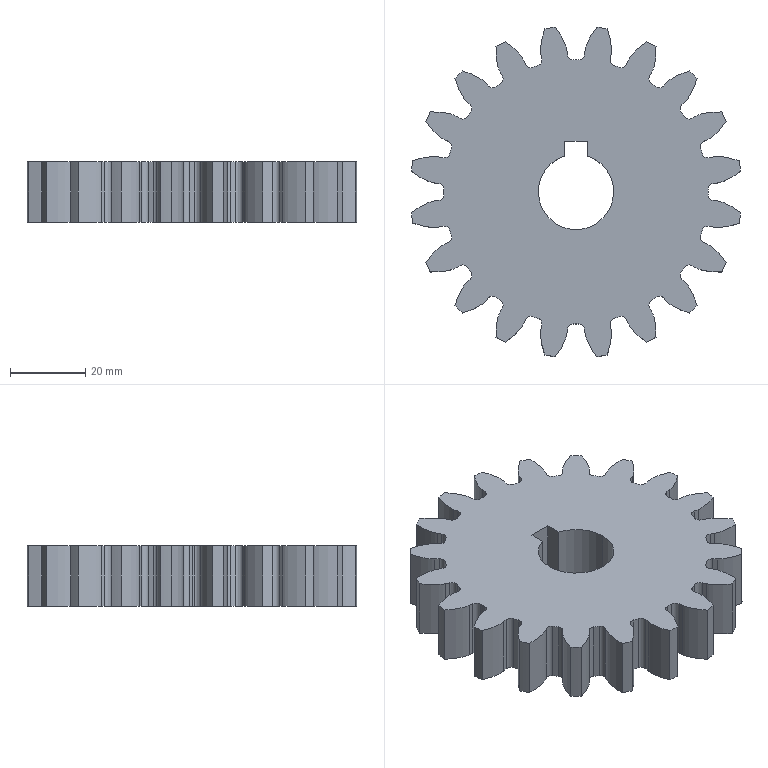Part | SolidWorks | features BaseBody 1 | 1 solid | 179 faces | box 87.308 x 87.308 x 16 mm | volume 73435 mm3 | cylinder 94 | plane 45 | spline 40 | commonest cylinder face diameters 3.04 x50 70 x21 88 x20 20 x3